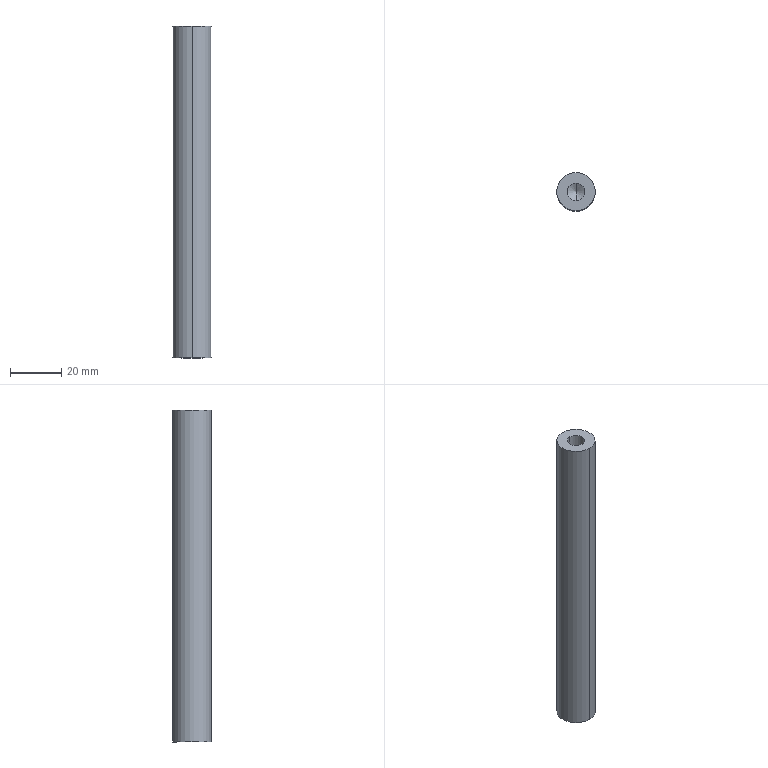Part | SolidWorks | features BaseBody 1 | 1 solid | 12 faces | box 15 x 15 x 130 mm | volume 21834 mm3 | cylinder 6 | cone 4 | plane 2 | commonest cylinder face diameters 6.8 x4 15 x2
STEP:
#1=CARTESIAN_POINT('',(-294.248,74.318,1.4));
#2=VERTEX_POINT('',#1);
#3=CARTESIAN_POINT('',(-294.248,89.318,1.4));
#4=VERTEX_POINT('',#3);
#5=CARTESIAN_POINT('',(-294.248,81.818,1.4));
#6=DIRECTION('',(0.,0.,1.));
#7=DIRECTION('',(0.,-1.,0.));
#8=AXIS2_PLACEMENT_3D('',#5,#6,#7);
#9=CIRCLE('',#8,7.5);
#10=EDGE_CURVE('',#2,#4,#9,.T.);
#11=ORIENTED_EDGE('',*,*,#10,.T.);
#12=CARTESIAN_POINT('',(-294.248,89.318,131.4));
#13=VERTEX_POINT('',#12);
#14=CARTESIAN_POINT('',(-294.248,89.318,1.4));
#15=DIRECTION('',(0.,0.,1.));
#16=VECTOR('',#15,1000.);
#17=LINE('',#14,#16);
#18=EDGE_CURVE('',#4,#13,#17,.T.);
#19=ORIENTED_EDGE('',*,*,#18,.T.);
#20=CARTESIAN_POINT('',(-294.248,74.318,131.4));
#21=VERTEX_POINT('',#20);
#22=CARTESIAN_POINT('',(-294.248,81.818,131.4));
#23=DIRECTION('',(0.,0.,-1.));
#24=DIRECTION('',(0.,-1.,0.));
#25=AXIS2_PLACEMENT_3D('',#22,#23,#24);
#26=CIRCLE('',#25,7.5);
#27=EDGE_CURVE('',#13,#21,#26,.T.);
#28=ORIENTED_EDGE('',*,*,#27,.T.);
#29=CARTESIAN_POINT('',(-294.248,74.318,1.4));
#30=DIRECTION('',(0.,0.,1.));
#31=VECTOR('',#30,1000.);
#32=LINE('',#29,#31);
#33=EDGE_CURVE('',#2,#21,#32,.T.);
#34=ORIENTED_EDGE('',*,*,#33,.F.);
#35=EDGE_LOOP('',(#11,#19,#28,#34));
#36=FACE_OUTER_BOUND('',#35,.T.);
#37=CARTESIAN_POINT('',(-294.248,81.818,1.4));
#38=DIRECTION('',(0.,0.,1.));
#39=DIRECTION('',(0.,-1.,0.));
#40=AXIS2_PLACEMENT_3D('',#37,#38,#39);
#41=CYLINDRICAL_SURFACE('',#40,7.5);
#42=ADVANCED_FACE('',(#36),#41,.T.);
#43=CARTESIAN_POINT('',(-294.248,85.218,116.4));
#44=VERTEX_POINT('',#43);
#45=CARTESIAN_POINT('',(-294.248,78.418,116.4));
#46=VERTEX_POINT('',#45);
#47=CARTESIAN_POINT('',(-294.248,81.818,116.4));
#48=DIRECTION('',(0.,0.,1.));
#49=DIRECTION('',(0.,-1.,0.));
#50=AXIS2_PLACEMENT_3D('',#47,#48,#49);
#51=CIRCLE('',#50,3.4);
#52=EDGE_CURVE('',#44,#46,#51,.T.);
#53=ORIENTED_EDGE('',*,*,#52,.F.);
#54=CARTESIAN_POINT('',(-294.248,85.218,131.4));
#55=VERTEX_POINT('',#54);
#56=CARTESIAN_POINT('',(-294.248,85.218,131.4));
#57=DIRECTION('',(0.,0.,1.));
#58=VECTOR('',#57,1000.);
#59=LINE('',#56,#58);
#60=EDGE_CURVE('',#44,#55,#59,.T.);
#61=ORIENTED_EDGE('',*,*,#60,.T.);
#62=CARTESIAN_POINT('',(-294.248,78.418,131.4));
#63=VERTEX_POINT('',#62);
#64=CARTESIAN_POINT('',(-294.248,81.818,131.4));
#65=DIRECTION('',(0.,0.,1.));
#66=DIRECTION('',(0.,-1.,0.));
#67=AXIS2_PLACEMENT_3D('',#64,#65,#66);
#68=CIRCLE('',#67,3.4);
#69=EDGE_CURVE('',#55,#63,#68,.T.);
#70=ORIENTED_EDGE('',*,*,#69,.T.);
#71=CARTESIAN_POINT('',(-294.248,78.418,131.4));
#72=DIRECTION('',(0.,0.,1.));
#73=VECTOR('',#72,1000.);
#74=LINE('',#71,#73);
#75=EDGE_CURVE('',#46,#63,#74,.T.);
#76=ORIENTED_EDGE('',*,*,#75,.F.);
#77=EDGE_LOOP('',(#53,#61,#70,#76));
#78=FACE_OUTER_BOUND('',#77,.T.);
#79=CARTESIAN_POINT('',(-294.248,81.818,131.4));
#80=DIRECTION('',(0.,0.,1.));
#81=DIRECTION('',(0.,-1.,0.));
#82=AXIS2_PLACEMENT_3D('',#79,#80,#81);
#83=CYLINDRICAL_SURFACE('',#82,3.4);
#84=ADVANCED_FACE('',(#78),#83,.F.);
#85=CARTESIAN_POINT('',(-294.248,78.418,16.4));
#86=VERTEX_POINT('',#85);
#87=CARTESIAN_POINT('',(-294.248,85.218,16.4));
#88=VERTEX_POINT('',#87);
#89=CARTESIAN_POINT('',(-294.248,81.818,16.4));
#90=DIRECTION('',(0.,0.,-1.));
#91=DIRECTION('',(0.,1.,0.));
#92=AXIS2_PLACEMENT_3D('',#89,#90,#91);
#93=CIRCLE('',#92,3.4);
#94=EDGE_CURVE('',#86,#88,#93,.T.);
#95=ORIENTED_EDGE('',*,*,#94,.F.);
#96=CARTESIAN_POINT('',(-294.248,78.418,1.4));
#97=VERTEX_POINT('',#96);
#98=CARTESIAN_POINT('',(-294.248,78.418,1.4));
#99=DIRECTION('',(0.,0.,-1.));
#100=VECTOR('',#99,1000.);
#101=LINE('',#98,#100);
#102=EDGE_CURVE('',#86,#97,#101,.T.);
#103=ORIENTED_EDGE('',*,*,#102,.T.);
#104=CARTESIAN_POINT('',(-294.248,85.218,1.4));
#105=VERTEX_POINT('',#104);
#106=CARTESIAN_POINT('',(-294.248,81.818,1.4));
#107=DIRECTION('',(0.,0.,1.));
#108=DIRECTION('',(0.,1.,0.));
#109=AXIS2_PLACEMENT_3D('',#106,#107,#108);
#110=CIRCLE('',#109,3.4);
#111=EDGE_CURVE('',#105,#97,#110,.T.);
#112=ORIENTED_EDGE('',*,*,#111,.F.);
#113=CARTESIAN_POINT('',(-294.248,85.218,1.4));
#114=DIRECTION('',(0.,0.,-1.));
#115=VECTOR('',#114,1000.);
#116=LINE('',#113,#115);
#117=EDGE_CURVE('',#88,#105,#116,.T.);
#118=ORIENTED_EDGE('',*,*,#117,.F.);
#119=EDGE_LOOP('',(#95,#103,#112,#118));
#120=FACE_OUTER_BOUND('',#119,.T.);
#121=CARTESIAN_POINT('',(-294.248,81.818,1.4));
#122=DIRECTION('',(0.,0.,-1.));
#123=DIRECTION('',(0.,1.,0.));
#124=AXIS2_PLACEMENT_3D('',#121,#122,#123);
#125=CYLINDRICAL_SURFACE('',#124,3.4);
#126=ADVANCED_FACE('',(#120),#125,.F.);
#127=CARTESIAN_POINT('',(-294.248,81.818,114.357));
#128=VERTEX_POINT('',#127);
#129=CARTESIAN_POINT('',(-294.248,78.418,116.4));
#130=DIRECTION('',(0.,-0.8572,0.515));
#131=VECTOR('',#130,1000.);
#132=LINE('',#129,#131);
#133=EDGE_CURVE('',#128,#46,#132,.T.);
#134=ORIENTED_EDGE('',*,*,#133,.F.);
#135=CARTESIAN_POINT('',(-294.248,85.218,116.4));
#136=DIRECTION('',(0.,0.8572,0.515));
#137=VECTOR('',#136,1000.);
#138=LINE('',#135,#137);
#139=EDGE_CURVE('',#128,#44,#138,.T.);
#140=ORIENTED_EDGE('',*,*,#139,.T.);
#141=ORIENTED_EDGE('',*,*,#52,.T.);
#142=EDGE_LOOP('',(#134,#140,#141));
#143=FACE_OUTER_BOUND('',#142,.T.);
#144=CARTESIAN_POINT('',(-294.248,81.818,116.4));
#145=DIRECTION('',(0.,0.,1.));
#146=DIRECTION('',(0.,-1.,0.));
#147=AXIS2_PLACEMENT_3D('',#144,#145,#146);
#148=CONICAL_SURFACE('',#147,3.4,1.03);
#149=ADVANCED_FACE('',(#143),#148,.F.);
#150=CARTESIAN_POINT('',(-294.248,81.818,18.443));
#151=VERTEX_POINT('',#150);
#152=CARTESIAN_POINT('',(-294.248,85.218,16.4));
#153=DIRECTION('',(0.,0.8572,-0.515));
#154=VECTOR('',#153,1000.);
#155=LINE('',#152,#154);
#156=EDGE_CURVE('',#151,#88,#155,.T.);
#157=ORIENTED_EDGE('',*,*,#156,.F.);
#158=CARTESIAN_POINT('',(-294.248,78.418,16.4));
#159=DIRECTION('',(0.,-0.8572,-0.515));
#160=VECTOR('',#159,1000.);
#161=LINE('',#158,#160);
#162=EDGE_CURVE('',#151,#86,#161,.T.);
#163=ORIENTED_EDGE('',*,*,#162,.T.);
#164=ORIENTED_EDGE('',*,*,#94,.T.);
#165=EDGE_LOOP('',(#157,#163,#164));
#166=FACE_OUTER_BOUND('',#165,.T.);
#167=CARTESIAN_POINT('',(-294.248,81.818,16.4));
#168=DIRECTION('',(0.,0.,-1.));
#169=DIRECTION('',(0.,1.,0.));
#170=AXIS2_PLACEMENT_3D('',#167,#168,#169);
#171=CONICAL_SURFACE('',#170,3.4,1.03);
#172=ADVANCED_FACE('',(#166),#171,.F.);
#173=ORIENTED_EDGE('',*,*,#18,.F.);
#174=CARTESIAN_POINT('',(-294.248,81.818,1.4));
#175=DIRECTION('',(0.,0.,1.));
#176=DIRECTION('',(0.,-1.,0.));
#177=AXIS2_PLACEMENT_3D('',#174,#175,#176);
#178=CIRCLE('',#177,7.5);
#179=EDGE_CURVE('',#4,#2,#178,.T.);
#180=ORIENTED_EDGE('',*,*,#179,.T.);
#181=ORIENTED_EDGE('',*,*,#33,.T.);
#182=CARTESIAN_POINT('',(-294.248,81.818,131.4));
#183=DIRECTION('',(0.,0.,-1.));
#184=DIRECTION('',(0.,-1.,0.));
#185=AXIS2_PLACEMENT_3D('',#182,#183,#184);
#186=CIRCLE('',#185,7.5);
#187=EDGE_CURVE('',#21,#13,#186,.T.);
#188=ORIENTED_EDGE('',*,*,#187,.T.);
#189=EDGE_LOOP('',(#173,#180,#181,#188));
#190=FACE_OUTER_BOUND('',#189,.T.);
#191=CARTESIAN_POINT('',(-294.248,81.818,1.4));
#192=DIRECTION('',(0.,0.,1.));
#193=DIRECTION('',(0.,-1.,0.));
#194=AXIS2_PLACEMENT_3D('',#191,#192,#193);
#195=CYLINDRICAL_SURFACE('',#194,7.5);
#196=ADVANCED_FACE('',(#190),#195,.T.);
#197=ORIENTED_EDGE('',*,*,#187,.F.);
#198=ORIENTED_EDGE('',*,*,#27,.F.);
#199=EDGE_LOOP('',(#197,#198));
#200=FACE_OUTER_BOUND('',#199,.T.);
#201=CARTESIAN_POINT('',(-294.248,81.818,131.4));
#202=DIRECTION('',(0.,0.,1.));
#203=DIRECTION('',(0.,-1.,0.));
#204=AXIS2_PLACEMENT_3D('',#201,#202,#203);
#205=CIRCLE('',#204,3.4);
#206=EDGE_CURVE('',#63,#55,#205,.T.);
#207=ORIENTED_EDGE('',*,*,#206,.F.);
#208=ORIENTED_EDGE('',*,*,#69,.F.);
#209=EDGE_LOOP('',(#207,#208));
#210=FACE_BOUND('',#209,.T.);
#211=CARTESIAN_POINT('',(-294.248,81.818,131.4));
#212=DIRECTION('',(0.,0.,-1.));
#213=DIRECTION('',(0.,1.,0.));
#214=AXIS2_PLACEMENT_3D('',#211,#212,#213);
#215=PLANE('',#214);
#216=ADVANCED_FACE('',(#200,#210),#215,.F.);
#217=ORIENTED_EDGE('',*,*,#10,.F.);
#218=ORIENTED_EDGE('',*,*,#179,.F.);
#219=EDGE_LOOP('',(#217,#218));
#220=FACE_OUTER_BOUND('',#219,.T.);
#221=ORIENTED_EDGE('',*,*,#111,.T.);
#222=CARTESIAN_POINT('',(-294.248,81.818,1.4));
#223=DIRECTION('',(0.,0.,1.));
#224=DIRECTION('',(0.,1.,0.));
#225=AXIS2_PLACEMENT_3D('',#222,#223,#224);
#226=CIRCLE('',#225,3.4);
#227=EDGE_CURVE('',#97,#105,#226,.T.);
#228=ORIENTED_EDGE('',*,*,#227,.T.);
#229=EDGE_LOOP('',(#221,#228));
#230=FACE_BOUND('',#229,.T.);
#231=CARTESIAN_POINT('',(-294.248,81.818,1.4));
#232=DIRECTION('',(0.,0.,-1.));
#233=DIRECTION('',(0.,1.,0.));
#234=AXIS2_PLACEMENT_3D('',#231,#232,#233);
#235=PLANE('',#234);
#236=ADVANCED_FACE('',(#220,#230),#235,.T.);
#237=ORIENTED_EDGE('',*,*,#60,.F.);
#238=CARTESIAN_POINT('',(-294.248,81.818,116.4));
#239=DIRECTION('',(0.,0.,1.));
#240=DIRECTION('',(0.,-1.,0.));
#241=AXIS2_PLACEMENT_3D('',#238,#239,#240);
#242=CIRCLE('',#241,3.4);
#243=EDGE_CURVE('',#46,#44,#242,.T.);
#244=ORIENTED_EDGE('',*,*,#243,.F.);
#245=ORIENTED_EDGE('',*,*,#75,.T.);
#246=ORIENTED_EDGE('',*,*,#206,.T.);
#247=EDGE_LOOP('',(#237,#244,#245,#246));
#248=FACE_OUTER_BOUND('',#247,.T.);
#249=CARTESIAN_POINT('',(-294.248,81.818,131.4));
#250=DIRECTION('',(0.,0.,1.));
#251=DIRECTION('',(0.,-1.,0.));
#252=AXIS2_PLACEMENT_3D('',#249,#250,#251);
#253=CYLINDRICAL_SURFACE('',#252,3.4);
#254=ADVANCED_FACE('',(#248),#253,.F.);
#255=ORIENTED_EDGE('',*,*,#102,.F.);
#256=CARTESIAN_POINT('',(-294.248,81.818,16.4));
#257=DIRECTION('',(0.,0.,-1.));
#258=DIRECTION('',(0.,1.,0.));
#259=AXIS2_PLACEMENT_3D('',#256,#257,#258);
#260=CIRCLE('',#259,3.4);
#261=EDGE_CURVE('',#88,#86,#260,.T.);
#262=ORIENTED_EDGE('',*,*,#261,.F.);
#263=ORIENTED_EDGE('',*,*,#117,.T.);
#264=ORIENTED_EDGE('',*,*,#227,.F.);
#265=EDGE_LOOP('',(#255,#262,#263,#264));
#266=FACE_OUTER_BOUND('',#265,.T.);
#267=CARTESIAN_POINT('',(-294.248,81.818,1.4));
#268=DIRECTION('',(0.,0.,-1.));
#269=DIRECTION('',(0.,1.,0.));
#270=AXIS2_PLACEMENT_3D('',#267,#268,#269);
#271=CYLINDRICAL_SURFACE('',#270,3.4);
#272=ADVANCED_FACE('',(#266),#271,.F.);
#273=ORIENTED_EDGE('',*,*,#139,.F.);
#274=ORIENTED_EDGE('',*,*,#133,.T.);
#275=ORIENTED_EDGE('',*,*,#243,.T.);
#276=EDGE_LOOP('',(#273,#274,#275));
#277=FACE_OUTER_BOUND('',#276,.T.);
#278=CARTESIAN_POINT('',(-294.248,81.818,116.4));
#279=DIRECTION('',(0.,0.,1.));
#280=DIRECTION('',(0.,-1.,0.));
#281=AXIS2_PLACEMENT_3D('',#278,#279,#280);
#282=CONICAL_SURFACE('',#281,3.4,1.03);
#283=ADVANCED_FACE('',(#277),#282,.F.);
#284=ORIENTED_EDGE('',*,*,#162,.F.);
#285=ORIENTED_EDGE('',*,*,#156,.T.);
#286=ORIENTED_EDGE('',*,*,#261,.T.);
#287=EDGE_LOOP('',(#284,#285,#286));
#288=FACE_OUTER_BOUND('',#287,.T.);
#289=CARTESIAN_POINT('',(-294.248,81.818,16.4));
#290=DIRECTION('',(0.,0.,-1.));
#291=DIRECTION('',(0.,1.,0.));
#292=AXIS2_PLACEMENT_3D('',#289,#290,#291);
#293=CONICAL_SURFACE('',#292,3.4,1.03);
#294=ADVANCED_FACE('',(#288),#293,.F.);
#295=CLOSED_SHELL('',(#42,#84,#126,#149,#172,#196,#216,#236,#254,#272,#283,#294));
#296=MANIFOLD_SOLID_BREP('',#295);
#297=CARTESIAN_POINT('',(0.,0.,0.));
#298=DIRECTION('',(0.,0.,1.));
#299=DIRECTION('',(1.,0.,0.));
#300=AXIS2_PLACEMENT_3D('',#297,#298,#299);
#301=(LENGTH_UNIT()NAMED_UNIT(*)SI_UNIT(.MILLI.,.METRE.));
#302=UNCERTAINTY_MEASURE_WITH_UNIT(LENGTH_MEASURE(0.00001),#301,'','');
#303=(NAMED_UNIT(*)PLANE_ANGLE_UNIT()SI_UNIT($,.RADIAN.));
#304=(NAMED_UNIT(*)SI_UNIT($,.STERADIAN.)SOLID_ANGLE_UNIT());
#305=(GEOMETRIC_REPRESENTATION_CONTEXT(3)GLOBAL_UNCERTAINTY_ASSIGNED_CONTEXT((#302))GLOBAL_UNIT_ASSIGNED_CONTEXT((#301,#303,#304))REPRESENTATION_CONTEXT('',''));
#306=ADVANCED_BREP_SHAPE_REPRESENTATION('',(#296,#300),#305);